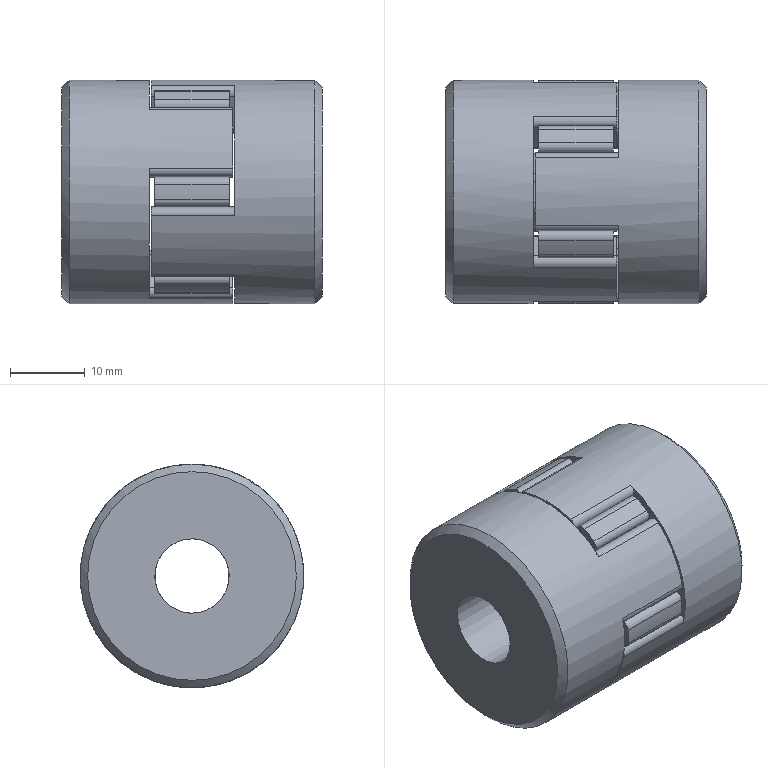Part | STEP file | YBQDJ-SSJ-11 | 1 solid | 121 faces | box 35 x 30 x 30 mm | volume 20965 mm3 | cylinder 71 | plane 48 | cone 2 | commonest cylinder face diameters 2 x48 16 x12 30 x8 10 x2 12 x1